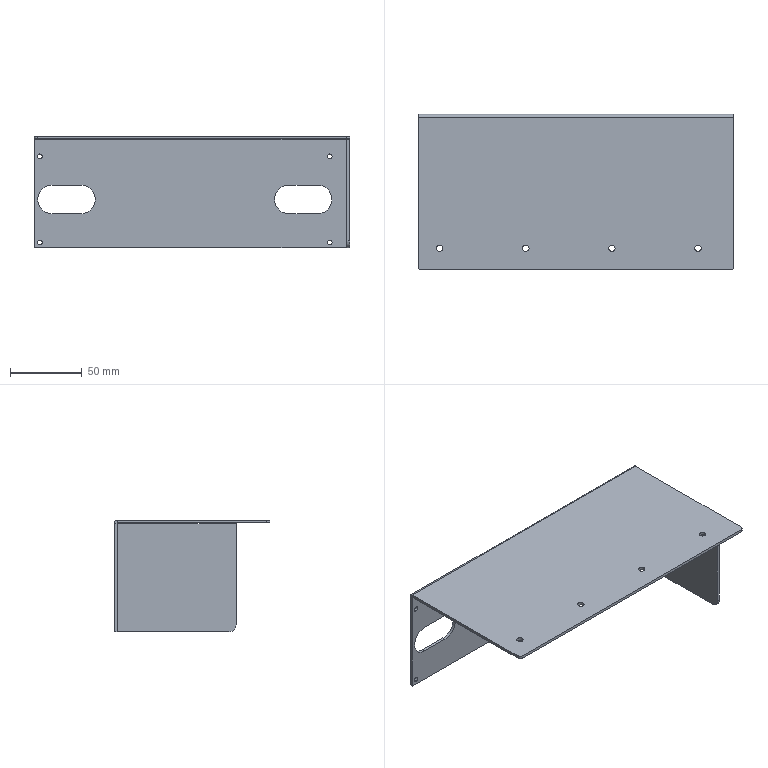Part | STEP file | push-button box mounting plate | 1 solid | 50 faces | box 220 x 108.5 x 78 mm | volume 90266 mm3 | cylinder 27 | plane 23 | commonest cylinder face diameters 3.3 x8 4.5 x8 20 x4 1 x2 4 x2 5 x2